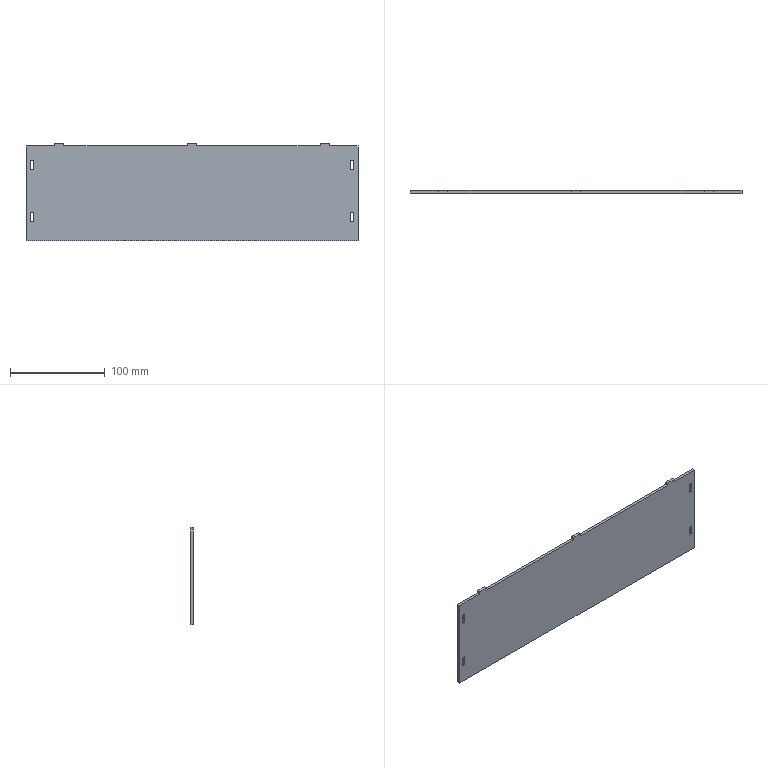Part | SolidWorks | features ICE 2, Extrusion 1 | 1 solid | 34 faces | box 350 x 3 x 103 mm | volume 104878 mm3 | plane 34
STEP:
#1=CARTESIAN_POINT('',(145.,3.,50.));
#2=VERTEX_POINT('',#1);
#3=CARTESIAN_POINT('',(175.,3.,50.));
#4=VERTEX_POINT('',#3);
#5=CARTESIAN_POINT('',(-175.,3.,50.));
#6=DIRECTION('',(1.,0.,0.));
#7=VECTOR('',#6,1000.);
#8=LINE('',#5,#7);
#9=EDGE_CURVE('',#2,#4,#8,.T.);
#10=ORIENTED_EDGE('',*,*,#9,.F.);
#11=CARTESIAN_POINT('',(145.,0.,50.));
#12=VERTEX_POINT('',#11);
#13=CARTESIAN_POINT('',(145.,-10.44,50.));
#14=DIRECTION('',(0.,1.,0.));
#15=VECTOR('',#14,1000.);
#16=LINE('',#13,#15);
#17=EDGE_CURVE('',#12,#2,#16,.T.);
#18=ORIENTED_EDGE('',*,*,#17,.F.);
#19=CARTESIAN_POINT('',(175.,0.,50.));
#20=VERTEX_POINT('',#19);
#21=CARTESIAN_POINT('',(-175.,0.,50.));
#22=DIRECTION('',(1.,0.,0.));
#23=VECTOR('',#22,1000.);
#24=LINE('',#21,#23);
#25=EDGE_CURVE('',#12,#20,#24,.T.);
#26=ORIENTED_EDGE('',*,*,#25,.T.);
#27=CARTESIAN_POINT('',(175.,3.,50.));
#28=DIRECTION('',(0.,-1.,0.));
#29=VECTOR('',#28,1000.);
#30=LINE('',#27,#29);
#31=EDGE_CURVE('',#4,#20,#30,.T.);
#32=ORIENTED_EDGE('',*,*,#31,.F.);
#33=EDGE_LOOP('',(#10,#18,#26,#32));
#34=FACE_OUTER_BOUND('',#33,.T.);
#35=CARTESIAN_POINT('',(-175.,3.,50.));
#36=DIRECTION('',(0.,0.,-1.));
#37=DIRECTION('',(-1.,0.,0.));
#38=AXIS2_PLACEMENT_3D('',#35,#36,#37);
#39=PLANE('',#38);
#40=ADVANCED_FACE('',(#34),#39,.F.);
#41=CARTESIAN_POINT('',(-135.,0.,50.));
#42=VERTEX_POINT('',#41);
#43=CARTESIAN_POINT('',(-5.,0.,50.));
#44=VERTEX_POINT('',#43);
#45=CARTESIAN_POINT('',(-175.,0.,50.));
#46=DIRECTION('',(1.,0.,0.));
#47=VECTOR('',#46,1000.);
#48=LINE('',#45,#47);
#49=EDGE_CURVE('',#42,#44,#48,.T.);
#50=ORIENTED_EDGE('',*,*,#49,.T.);
#51=CARTESIAN_POINT('',(-5.,3.,50.));
#52=VERTEX_POINT('',#51);
#53=CARTESIAN_POINT('',(-5.,-10.44,50.));
#54=DIRECTION('',(0.,1.,0.));
#55=VECTOR('',#54,1000.);
#56=LINE('',#53,#55);
#57=EDGE_CURVE('',#44,#52,#56,.T.);
#58=ORIENTED_EDGE('',*,*,#57,.T.);
#59=CARTESIAN_POINT('',(-135.,3.,50.));
#60=VERTEX_POINT('',#59);
#61=CARTESIAN_POINT('',(-175.,3.,50.));
#62=DIRECTION('',(1.,0.,0.));
#63=VECTOR('',#62,1000.);
#64=LINE('',#61,#63);
#65=EDGE_CURVE('',#60,#52,#64,.T.);
#66=ORIENTED_EDGE('',*,*,#65,.F.);
#67=CARTESIAN_POINT('',(-135.,-10.44,50.));
#68=DIRECTION('',(0.,1.,0.));
#69=VECTOR('',#68,1000.);
#70=LINE('',#67,#69);
#71=EDGE_CURVE('',#42,#60,#70,.T.);
#72=ORIENTED_EDGE('',*,*,#71,.F.);
#73=EDGE_LOOP('',(#50,#58,#66,#72));
#74=FACE_OUTER_BOUND('',#73,.T.);
#75=CARTESIAN_POINT('',(-175.,3.,50.));
#76=DIRECTION('',(0.,0.,-1.));
#77=DIRECTION('',(-1.,0.,0.));
#78=AXIS2_PLACEMENT_3D('',#75,#76,#77);
#79=PLANE('',#78);
#80=ADVANCED_FACE('',(#74),#79,.F.);
#81=CARTESIAN_POINT('',(5.,0.,50.));
#82=VERTEX_POINT('',#81);
#83=CARTESIAN_POINT('',(135.,0.,50.));
#84=VERTEX_POINT('',#83);
#85=CARTESIAN_POINT('',(-175.,0.,50.));
#86=DIRECTION('',(1.,0.,0.));
#87=VECTOR('',#86,1000.);
#88=LINE('',#85,#87);
#89=EDGE_CURVE('',#82,#84,#88,.T.);
#90=ORIENTED_EDGE('',*,*,#89,.T.);
#91=CARTESIAN_POINT('',(135.,3.,50.));
#92=VERTEX_POINT('',#91);
#93=CARTESIAN_POINT('',(135.,-10.44,50.));
#94=DIRECTION('',(0.,1.,0.));
#95=VECTOR('',#94,1000.);
#96=LINE('',#93,#95);
#97=EDGE_CURVE('',#84,#92,#96,.T.);
#98=ORIENTED_EDGE('',*,*,#97,.T.);
#99=CARTESIAN_POINT('',(5.,3.,50.));
#100=VERTEX_POINT('',#99);
#101=CARTESIAN_POINT('',(-175.,3.,50.));
#102=DIRECTION('',(1.,0.,0.));
#103=VECTOR('',#102,1000.);
#104=LINE('',#101,#103);
#105=EDGE_CURVE('',#100,#92,#104,.T.);
#106=ORIENTED_EDGE('',*,*,#105,.F.);
#107=CARTESIAN_POINT('',(5.,-10.44,50.));
#108=DIRECTION('',(0.,1.,0.));
#109=VECTOR('',#108,1000.);
#110=LINE('',#107,#109);
#111=EDGE_CURVE('',#82,#100,#110,.T.);
#112=ORIENTED_EDGE('',*,*,#111,.F.);
#113=EDGE_LOOP('',(#90,#98,#106,#112));
#114=FACE_OUTER_BOUND('',#113,.T.);
#115=CARTESIAN_POINT('',(-175.,3.,50.));
#116=DIRECTION('',(0.,0.,-1.));
#117=DIRECTION('',(-1.,0.,0.));
#118=AXIS2_PLACEMENT_3D('',#115,#116,#117);
#119=PLANE('',#118);
#120=ADVANCED_FACE('',(#114),#119,.F.);
#121=CARTESIAN_POINT('',(175.,0.,-50.));
#122=VERTEX_POINT('',#121);
#123=CARTESIAN_POINT('',(175.,0.,50.));
#124=DIRECTION('',(0.,0.,-1.));
#125=VECTOR('',#124,1000.);
#126=LINE('',#123,#125);
#127=EDGE_CURVE('',#20,#122,#126,.T.);
#128=ORIENTED_EDGE('',*,*,#127,.T.);
#129=CARTESIAN_POINT('',(175.,3.,-50.));
#130=VERTEX_POINT('',#129);
#131=CARTESIAN_POINT('',(175.,3.,-50.));
#132=DIRECTION('',(0.,-1.,0.));
#133=VECTOR('',#132,1000.);
#134=LINE('',#131,#133);
#135=EDGE_CURVE('',#130,#122,#134,.T.);
#136=ORIENTED_EDGE('',*,*,#135,.F.);
#137=CARTESIAN_POINT('',(175.,3.,50.));
#138=DIRECTION('',(0.,0.,-1.));
#139=VECTOR('',#138,1000.);
#140=LINE('',#137,#139);
#141=EDGE_CURVE('',#4,#130,#140,.T.);
#142=ORIENTED_EDGE('',*,*,#141,.F.);
#143=ORIENTED_EDGE('',*,*,#31,.T.);
#144=EDGE_LOOP('',(#128,#136,#142,#143));
#145=FACE_OUTER_BOUND('',#144,.T.);
#146=CARTESIAN_POINT('',(175.,3.,50.));
#147=DIRECTION('',(-1.,0.,0.));
#148=DIRECTION('',(0.,0.,1.));
#149=AXIS2_PLACEMENT_3D('',#146,#147,#148);
#150=PLANE('',#149);
#151=ADVANCED_FACE('',(#145),#150,.F.);
#152=CARTESIAN_POINT('',(-175.,0.,-50.));
#153=VERTEX_POINT('',#152);
#154=CARTESIAN_POINT('',(-175.,0.,-50.));
#155=DIRECTION('',(-1.,0.,0.));
#156=VECTOR('',#155,1000.);
#157=LINE('',#154,#156);
#158=EDGE_CURVE('',#122,#153,#157,.T.);
#159=ORIENTED_EDGE('',*,*,#158,.T.);
#160=CARTESIAN_POINT('',(-175.,3.,-50.));
#161=VERTEX_POINT('',#160);
#162=CARTESIAN_POINT('',(-175.,3.,-50.));
#163=DIRECTION('',(0.,-1.,0.));
#164=VECTOR('',#163,1000.);
#165=LINE('',#162,#164);
#166=EDGE_CURVE('',#161,#153,#165,.T.);
#167=ORIENTED_EDGE('',*,*,#166,.F.);
#168=CARTESIAN_POINT('',(-175.,3.,-50.));
#169=DIRECTION('',(-1.,0.,0.));
#170=VECTOR('',#169,1000.);
#171=LINE('',#168,#170);
#172=EDGE_CURVE('',#130,#161,#171,.T.);
#173=ORIENTED_EDGE('',*,*,#172,.F.);
#174=ORIENTED_EDGE('',*,*,#135,.T.);
#175=EDGE_LOOP('',(#159,#167,#173,#174));
#176=FACE_OUTER_BOUND('',#175,.T.);
#177=CARTESIAN_POINT('',(-175.,3.,-50.));
#178=DIRECTION('',(0.,0.,1.));
#179=DIRECTION('',(1.,0.,0.));
#180=AXIS2_PLACEMENT_3D('',#177,#178,#179);
#181=PLANE('',#180);
#182=ADVANCED_FACE('',(#176),#181,.F.);
#183=CARTESIAN_POINT('',(-175.,0.,50.));
#184=VERTEX_POINT('',#183);
#185=CARTESIAN_POINT('',(-175.,0.,50.));
#186=DIRECTION('',(0.,0.,1.));
#187=VECTOR('',#186,1000.);
#188=LINE('',#185,#187);
#189=EDGE_CURVE('',#153,#184,#188,.T.);
#190=ORIENTED_EDGE('',*,*,#189,.T.);
#191=CARTESIAN_POINT('',(-175.,3.,50.));
#192=VERTEX_POINT('',#191);
#193=CARTESIAN_POINT('',(-175.,3.,50.));
#194=DIRECTION('',(0.,-1.,0.));
#195=VECTOR('',#194,1000.);
#196=LINE('',#193,#195);
#197=EDGE_CURVE('',#192,#184,#196,.T.);
#198=ORIENTED_EDGE('',*,*,#197,.F.);
#199=CARTESIAN_POINT('',(-175.,3.,50.));
#200=DIRECTION('',(0.,0.,1.));
#201=VECTOR('',#200,1000.);
#202=LINE('',#199,#201);
#203=EDGE_CURVE('',#161,#192,#202,.T.);
#204=ORIENTED_EDGE('',*,*,#203,.F.);
#205=ORIENTED_EDGE('',*,*,#166,.T.);
#206=EDGE_LOOP('',(#190,#198,#204,#205));
#207=FACE_OUTER_BOUND('',#206,.T.);
#208=CARTESIAN_POINT('',(-175.,3.,50.));
#209=DIRECTION('',(1.,0.,0.));
#210=DIRECTION('',(0.,0.,-1.));
#211=AXIS2_PLACEMENT_3D('',#208,#209,#210);
#212=PLANE('',#211);
#213=ADVANCED_FACE('',(#207),#212,.F.);
#214=CARTESIAN_POINT('',(-145.,0.,50.));
#215=VERTEX_POINT('',#214);
#216=CARTESIAN_POINT('',(-175.,0.,50.));
#217=DIRECTION('',(1.,0.,0.));
#218=VECTOR('',#217,1000.);
#219=LINE('',#216,#218);
#220=EDGE_CURVE('',#184,#215,#219,.T.);
#221=ORIENTED_EDGE('',*,*,#220,.T.);
#222=CARTESIAN_POINT('',(-145.,3.,50.));
#223=VERTEX_POINT('',#222);
#224=CARTESIAN_POINT('',(-145.,-10.44,50.));
#225=DIRECTION('',(0.,1.,0.));
#226=VECTOR('',#225,1000.);
#227=LINE('',#224,#226);
#228=EDGE_CURVE('',#215,#223,#227,.T.);
#229=ORIENTED_EDGE('',*,*,#228,.T.);
#230=CARTESIAN_POINT('',(-175.,3.,50.));
#231=DIRECTION('',(1.,0.,0.));
#232=VECTOR('',#231,1000.);
#233=LINE('',#230,#232);
#234=EDGE_CURVE('',#192,#223,#233,.T.);
#235=ORIENTED_EDGE('',*,*,#234,.F.);
#236=ORIENTED_EDGE('',*,*,#197,.T.);
#237=EDGE_LOOP('',(#221,#229,#235,#236));
#238=FACE_OUTER_BOUND('',#237,.T.);
#239=CARTESIAN_POINT('',(-175.,3.,50.));
#240=DIRECTION('',(0.,0.,-1.));
#241=DIRECTION('',(-1.,0.,0.));
#242=AXIS2_PLACEMENT_3D('',#239,#240,#241);
#243=PLANE('',#242);
#244=ADVANCED_FACE('',(#238),#243,.F.);
#245=CARTESIAN_POINT('',(167.4,3.,-30.1));
#246=VERTEX_POINT('',#245);
#247=CARTESIAN_POINT('',(167.4,3.,-19.9));
#248=VERTEX_POINT('',#247);
#249=CARTESIAN_POINT('',(167.4,3.,-30.1));
#250=DIRECTION('',(0.,0.,1.));
#251=VECTOR('',#250,1000.);
#252=LINE('',#249,#251);
#253=EDGE_CURVE('',#246,#248,#252,.T.);
#254=ORIENTED_EDGE('',*,*,#253,.F.);
#255=CARTESIAN_POINT('',(170.6,3.,-30.1));
#256=VERTEX_POINT('',#255);
#257=CARTESIAN_POINT('',(170.6,3.,-30.1));
#258=DIRECTION('',(-1.,0.,0.));
#259=VECTOR('',#258,1000.);
#260=LINE('',#257,#259);
#261=EDGE_CURVE('',#256,#246,#260,.T.);
#262=ORIENTED_EDGE('',*,*,#261,.F.);
#263=CARTESIAN_POINT('',(170.6,3.,-19.9));
#264=VERTEX_POINT('',#263);
#265=CARTESIAN_POINT('',(170.6,3.,-30.1));
#266=DIRECTION('',(0.,0.,-1.));
#267=VECTOR('',#266,1000.);
#268=LINE('',#265,#267);
#269=EDGE_CURVE('',#264,#256,#268,.T.);
#270=ORIENTED_EDGE('',*,*,#269,.F.);
#271=CARTESIAN_POINT('',(170.6,3.,-19.9));
#272=DIRECTION('',(1.,0.,0.));
#273=VECTOR('',#272,1000.);
#274=LINE('',#271,#273);
#275=EDGE_CURVE('',#248,#264,#274,.T.);
#276=ORIENTED_EDGE('',*,*,#275,.F.);
#277=EDGE_LOOP('',(#254,#262,#270,#276));
#278=FACE_BOUND('',#277,.T.);
#279=CARTESIAN_POINT('',(167.4,3.,24.9));
#280=VERTEX_POINT('',#279);
#281=CARTESIAN_POINT('',(167.4,3.,35.1));
#282=VERTEX_POINT('',#281);
#283=CARTESIAN_POINT('',(167.4,3.,24.9));
#284=DIRECTION('',(0.,0.,1.));
#285=VECTOR('',#284,1000.);
#286=LINE('',#283,#285);
#287=EDGE_CURVE('',#280,#282,#286,.T.);
#288=ORIENTED_EDGE('',*,*,#287,.F.);
#289=CARTESIAN_POINT('',(170.6,3.,24.9));
#290=VERTEX_POINT('',#289);
#291=CARTESIAN_POINT('',(170.6,3.,24.9));
#292=DIRECTION('',(-1.,0.,0.));
#293=VECTOR('',#292,1000.);
#294=LINE('',#291,#293);
#295=EDGE_CURVE('',#290,#280,#294,.T.);
#296=ORIENTED_EDGE('',*,*,#295,.F.);
#297=CARTESIAN_POINT('',(170.6,3.,35.1));
#298=VERTEX_POINT('',#297);
#299=CARTESIAN_POINT('',(170.6,3.,24.9));
#300=DIRECTION('',(0.,0.,-1.));
#301=VECTOR('',#300,1000.);
#302=LINE('',#299,#301);
#303=EDGE_CURVE('',#298,#290,#302,.T.);
#304=ORIENTED_EDGE('',*,*,#303,.F.);
#305=CARTESIAN_POINT('',(170.6,3.,35.1));
#306=DIRECTION('',(1.,0.,0.));
#307=VECTOR('',#306,1000.);
#308=LINE('',#305,#307);
#309=EDGE_CURVE('',#282,#298,#308,.T.);
#310=ORIENTED_EDGE('',*,*,#309,.F.);
#311=EDGE_LOOP('',(#288,#296,#304,#310));
#312=FACE_BOUND('',#311,.T.);
#313=CARTESIAN_POINT('',(-170.6,3.,35.1));
#314=VERTEX_POINT('',#313);
#315=CARTESIAN_POINT('',(-167.4,3.,35.1));
#316=VERTEX_POINT('',#315);
#317=CARTESIAN_POINT('',(-170.6,3.,35.1));
#318=DIRECTION('',(1.,0.,0.));
#319=VECTOR('',#318,1000.);
#320=LINE('',#317,#319);
#321=EDGE_CURVE('',#314,#316,#320,.T.);
#322=ORIENTED_EDGE('',*,*,#321,.F.);
#323=CARTESIAN_POINT('',(-170.6,3.,24.9));
#324=VERTEX_POINT('',#323);
#325=CARTESIAN_POINT('',(-170.6,3.,24.9));
#326=DIRECTION('',(0.,0.,1.));
#327=VECTOR('',#326,1000.);
#328=LINE('',#325,#327);
#329=EDGE_CURVE('',#324,#314,#328,.T.);
#330=ORIENTED_EDGE('',*,*,#329,.F.);
#331=CARTESIAN_POINT('',(-167.4,3.,24.9));
#332=VERTEX_POINT('',#331);
#333=CARTESIAN_POINT('',(-170.6,3.,24.9));
#334=DIRECTION('',(-1.,0.,0.));
#335=VECTOR('',#334,1000.);
#336=LINE('',#333,#335);
#337=EDGE_CURVE('',#332,#324,#336,.T.);
#338=ORIENTED_EDGE('',*,*,#337,.F.);
#339=CARTESIAN_POINT('',(-167.4,3.,24.9));
#340=DIRECTION('',(0.,0.,-1.));
#341=VECTOR('',#340,1000.);
#342=LINE('',#339,#341);
#343=EDGE_CURVE('',#316,#332,#342,.T.);
#344=ORIENTED_EDGE('',*,*,#343,.F.);
#345=EDGE_LOOP('',(#322,#330,#338,#344));
#346=FACE_BOUND('',#345,.T.);
#347=CARTESIAN_POINT('',(-170.6,3.,-19.9));
#348=VERTEX_POINT('',#347);
#349=CARTESIAN_POINT('',(-167.4,3.,-19.9));
#350=VERTEX_POINT('',#349);
#351=CARTESIAN_POINT('',(-170.6,3.,-19.9));
#352=DIRECTION('',(1.,0.,0.));
#353=VECTOR('',#352,1000.);
#354=LINE('',#351,#353);
#355=EDGE_CURVE('',#348,#350,#354,.T.);
#356=ORIENTED_EDGE('',*,*,#355,.F.);
#357=CARTESIAN_POINT('',(-170.6,3.,-30.1));
#358=VERTEX_POINT('',#357);
#359=CARTESIAN_POINT('',(-170.6,3.,-30.1));
#360=DIRECTION('',(0.,0.,1.));
#361=VECTOR('',#360,1000.);
#362=LINE('',#359,#361);
#363=EDGE_CURVE('',#358,#348,#362,.T.);
#364=ORIENTED_EDGE('',*,*,#363,.F.);
#365=CARTESIAN_POINT('',(-167.4,3.,-30.1));
#366=VERTEX_POINT('',#365);
#367=CARTESIAN_POINT('',(-170.6,3.,-30.1));
#368=DIRECTION('',(-1.,0.,0.));
#369=VECTOR('',#368,1000.);
#370=LINE('',#367,#369);
#371=EDGE_CURVE('',#366,#358,#370,.T.);
#372=ORIENTED_EDGE('',*,*,#371,.F.);
#373=CARTESIAN_POINT('',(-167.4,3.,-30.1));
#374=DIRECTION('',(0.,0.,-1.));
#375=VECTOR('',#374,1000.);
#376=LINE('',#373,#375);
#377=EDGE_CURVE('',#350,#366,#376,.T.);
#378=ORIENTED_EDGE('',*,*,#377,.F.);
#379=EDGE_LOOP('',(#356,#364,#372,#378));
#380=FACE_BOUND('',#379,.T.);
#381=ORIENTED_EDGE('',*,*,#141,.T.);
#382=ORIENTED_EDGE('',*,*,#172,.T.);
#383=ORIENTED_EDGE('',*,*,#203,.T.);
#384=ORIENTED_EDGE('',*,*,#234,.T.);
#385=CARTESIAN_POINT('',(-145.,3.,53.));
#386=VERTEX_POINT('',#385);
#387=CARTESIAN_POINT('',(-145.,3.,50.));
#388=DIRECTION('',(0.,0.,1.));
#389=VECTOR('',#388,1000.);
#390=LINE('',#387,#389);
#391=EDGE_CURVE('',#223,#386,#390,.T.);
#392=ORIENTED_EDGE('',*,*,#391,.T.);
#393=CARTESIAN_POINT('',(-135.,3.,53.));
#394=VERTEX_POINT('',#393);
#395=CARTESIAN_POINT('',(-145.,3.,53.));
#396=DIRECTION('',(1.,0.,0.));
#397=VECTOR('',#396,1000.);
#398=LINE('',#395,#397);
#399=EDGE_CURVE('',#386,#394,#398,.T.);
#400=ORIENTED_EDGE('',*,*,#399,.T.);
#401=CARTESIAN_POINT('',(-135.,3.,50.));
#402=DIRECTION('',(0.,0.,-1.));
#403=VECTOR('',#402,1000.);
#404=LINE('',#401,#403);
#405=EDGE_CURVE('',#394,#60,#404,.T.);
#406=ORIENTED_EDGE('',*,*,#405,.T.);
#407=ORIENTED_EDGE('',*,*,#65,.T.);
#408=CARTESIAN_POINT('',(-5.,3.,53.));
#409=VERTEX_POINT('',#408);
#410=CARTESIAN_POINT('',(-5.,3.,53.));
#411=DIRECTION('',(0.,0.,1.));
#412=VECTOR('',#411,1000.);
#413=LINE('',#410,#412);
#414=EDGE_CURVE('',#52,#409,#413,.T.);
#415=ORIENTED_EDGE('',*,*,#414,.T.);
#416=CARTESIAN_POINT('',(5.,3.,53.));
#417=VERTEX_POINT('',#416);
#418=CARTESIAN_POINT('',(-5.,3.,53.));
#419=DIRECTION('',(1.,0.,0.));
#420=VECTOR('',#419,1000.);
#421=LINE('',#418,#420);
#422=EDGE_CURVE('',#409,#417,#421,.T.);
#423=ORIENTED_EDGE('',*,*,#422,.T.);
#424=CARTESIAN_POINT('',(5.,3.,53.));
#425=DIRECTION('',(0.,0.,-1.));
#426=VECTOR('',#425,1000.);
#427=LINE('',#424,#426);
#428=EDGE_CURVE('',#417,#100,#427,.T.);
#429=ORIENTED_EDGE('',*,*,#428,.T.);
#430=ORIENTED_EDGE('',*,*,#105,.T.);
#431=CARTESIAN_POINT('',(135.,3.,53.));
#432=VERTEX_POINT('',#431);
#433=CARTESIAN_POINT('',(135.,3.,50.));
#434=DIRECTION('',(0.,0.,1.));
#435=VECTOR('',#434,1000.);
#436=LINE('',#433,#435);
#437=EDGE_CURVE('',#92,#432,#436,.T.);
#438=ORIENTED_EDGE('',*,*,#437,.T.);
#439=CARTESIAN_POINT('',(145.,3.,53.));
#440=VERTEX_POINT('',#439);
#441=CARTESIAN_POINT('',(135.,3.,53.));
#442=DIRECTION('',(1.,0.,0.));
#443=VECTOR('',#442,1000.);
#444=LINE('',#441,#443);
#445=EDGE_CURVE('',#432,#440,#444,.T.);
#446=ORIENTED_EDGE('',*,*,#445,.T.);
#447=CARTESIAN_POINT('',(145.,3.,50.));
#448=DIRECTION('',(0.,0.,-1.));
#449=VECTOR('',#448,1000.);
#450=LINE('',#447,#449);
#451=EDGE_CURVE('',#440,#2,#450,.T.);
#452=ORIENTED_EDGE('',*,*,#451,.T.);
#453=ORIENTED_EDGE('',*,*,#9,.T.);
#454=EDGE_LOOP('',(#381,#382,#383,#384,#392,#400,#406,#407,#415,#423,#429,#430,#438,#446,#452,#453));
#455=FACE_OUTER_BOUND('',#454,.T.);
#456=CARTESIAN_POINT('',(0.,3.,0.));
#457=DIRECTION('',(0.,-1.,0.));
#458=DIRECTION('',(0.,0.,-1.));
#459=AXIS2_PLACEMENT_3D('',#456,#457,#458);
#460=PLANE('',#459);
#461=ADVANCED_FACE('',(#278,#312,#346,#380,#455),#460,.F.);
#462=CARTESIAN_POINT('',(170.6,0.,-30.1));
#463=VERTEX_POINT('',#462);
#464=CARTESIAN_POINT('',(167.4,0.,-30.1));
#465=VERTEX_POINT('',#464);
#466=CARTESIAN_POINT('',(170.6,0.,-30.1));
#467=DIRECTION('',(-1.,0.,0.));
#468=VECTOR('',#467,1000.);
#469=LINE('',#466,#468);
#470=EDGE_CURVE('',#463,#465,#469,.T.);
#471=ORIENTED_EDGE('',*,*,#470,.T.);
#472=CARTESIAN_POINT('',(167.4,0.,-19.9));
#473=VERTEX_POINT('',#472);
#474=CARTESIAN_POINT('',(167.4,0.,-30.1));
#475=DIRECTION('',(0.,0.,1.));
#476=VECTOR('',#475,1000.);
#477=LINE('',#474,#476);
#478=EDGE_CURVE('',#465,#473,#477,.T.);
#479=ORIENTED_EDGE('',*,*,#478,.T.);
#480=CARTESIAN_POINT('',(170.6,0.,-19.9));
#481=VERTEX_POINT('',#480);
#482=CARTESIAN_POINT('',(170.6,0.,-19.9));
#483=DIRECTION('',(1.,0.,0.));
#484=VECTOR('',#483,1000.);
#485=LINE('',#482,#484);
#486=EDGE_CURVE('',#473,#481,#485,.T.);
#487=ORIENTED_EDGE('',*,*,#486,.T.);
#488=CARTESIAN_POINT('',(170.6,0.,-30.1));
#489=DIRECTION('',(0.,0.,-1.));
#490=VECTOR('',#489,1000.);
#491=LINE('',#488,#490);
#492=EDGE_CURVE('',#481,#463,#491,.T.);
#493=ORIENTED_EDGE('',*,*,#492,.T.);
#494=EDGE_LOOP('',(#471,#479,#487,#493));
#495=FACE_BOUND('',#494,.T.);
#496=CARTESIAN_POINT('',(170.6,0.,24.9));
#497=VERTEX_POINT('',#496);
#498=CARTESIAN_POINT('',(167.4,0.,24.9));
#499=VERTEX_POINT('',#498);
#500=CARTESIAN_POINT('',(170.6,0.,24.9));
#501=DIRECTION('',(-1.,0.,0.));
#502=VECTOR('',#501,1000.);
#503=LINE('',#500,#502);
#504=EDGE_CURVE('',#497,#499,#503,.T.);
#505=ORIENTED_EDGE('',*,*,#504,.T.);
#506=CARTESIAN_POINT('',(167.4,0.,35.1));
#507=VERTEX_POINT('',#506);
#508=CARTESIAN_POINT('',(167.4,0.,24.9));
#509=DIRECTION('',(0.,0.,1.));
#510=VECTOR('',#509,1000.);
#511=LINE('',#508,#510);
#512=EDGE_CURVE('',#499,#507,#511,.T.);
#513=ORIENTED_EDGE('',*,*,#512,.T.);
#514=CARTESIAN_POINT('',(170.6,0.,35.1));
#515=VERTEX_POINT('',#514);
#516=CARTESIAN_POINT('',(170.6,0.,35.1));
#517=DIRECTION('',(1.,0.,0.));
#518=VECTOR('',#517,1000.);
#519=LINE('',#516,#518);
#520=EDGE_CURVE('',#507,#515,#519,.T.);
#521=ORIENTED_EDGE('',*,*,#520,.T.);
#522=CARTESIAN_POINT('',(170.6,0.,24.9));
#523=DIRECTION('',(0.,0.,-1.));
#524=VECTOR('',#523,1000.);
#525=LINE('',#522,#524);
#526=EDGE_CURVE('',#515,#497,#525,.T.);
#527=ORIENTED_EDGE('',*,*,#526,.T.);
#528=EDGE_LOOP('',(#505,#513,#521,#527));
#529=FACE_BOUND('',#528,.T.);
#530=CARTESIAN_POINT('',(-170.6,0.,24.9));
#531=VERTEX_POINT('',#530);
#532=CARTESIAN_POINT('',(-170.6,0.,35.1));
#533=VERTEX_POINT('',#532);
#534=CARTESIAN_POINT('',(-170.6,0.,24.9));
#535=DIRECTION('',(0.,0.,1.));
#536=VECTOR('',#535,1000.);
#537=LINE('',#534,#536);
#538=EDGE_CURVE('',#531,#533,#537,.T.);
#539=ORIENTED_EDGE('',*,*,#538,.T.);
#540=CARTESIAN_POINT('',(-167.4,0.,35.1));
#541=VERTEX_POINT('',#540);
#542=CARTESIAN_POINT('',(-170.6,0.,35.1));
#543=DIRECTION('',(1.,0.,0.));
#544=VECTOR('',#543,1000.);
#545=LINE('',#542,#544);
#546=EDGE_CURVE('',#533,#541,#545,.T.);
#547=ORIENTED_EDGE('',*,*,#546,.T.);
#548=CARTESIAN_POINT('',(-167.4,0.,24.9));
#549=VERTEX_POINT('',#548);
#550=CARTESIAN_POINT('',(-167.4,0.,24.9));
#551=DIRECTION('',(0.,0.,-1.));
#552=VECTOR('',#551,1000.);
#553=LINE('',#550,#552);
#554=EDGE_CURVE('',#541,#549,#553,.T.);
#555=ORIENTED_EDGE('',*,*,#554,.T.);
#556=CARTESIAN_POINT('',(-170.6,0.,24.9));
#557=DIRECTION('',(-1.,0.,0.));
#558=VECTOR('',#557,1000.);
#559=LINE('',#556,#558);
#560=EDGE_CURVE('',#549,#531,#559,.T.);
#561=ORIENTED_EDGE('',*,*,#560,.T.);
#562=EDGE_LOOP('',(#539,#547,#555,#561));
#563=FACE_BOUND('',#562,.T.);
#564=CARTESIAN_POINT('',(-170.6,0.,-30.1));
#565=VERTEX_POINT('',#564);
#566=CARTESIAN_POINT('',(-170.6,0.,-19.9));
#567=VERTEX_POINT('',#566);
#568=CARTESIAN_POINT('',(-170.6,0.,-30.1));
#569=DIRECTION('',(0.,0.,1.));
#570=VECTOR('',#569,1000.);
#571=LINE('',#568,#570);
#572=EDGE_CURVE('',#565,#567,#571,.T.);
#573=ORIENTED_EDGE('',*,*,#572,.T.);
#574=CARTESIAN_POINT('',(-167.4,0.,-19.9));
#575=VERTEX_POINT('',#574);
#576=CARTESIAN_POINT('',(-170.6,0.,-19.9));
#577=DIRECTION('',(1.,0.,0.));
#578=VECTOR('',#577,1000.);
#579=LINE('',#576,#578);
#580=EDGE_CURVE('',#567,#575,#579,.T.);
#581=ORIENTED_EDGE('',*,*,#580,.T.);
#582=CARTESIAN_POINT('',(-167.4,0.,-30.1));
#583=VERTEX_POINT('',#582);
#584=CARTESIAN_POINT('',(-167.4,0.,-30.1));
#585=DIRECTION('',(0.,0.,-1.));
#586=VECTOR('',#585,1000.);
#587=LINE('',#584,#586);
#588=EDGE_CURVE('',#575,#583,#587,.T.);
#589=ORIENTED_EDGE('',*,*,#588,.T.);
#590=CARTESIAN_POINT('',(-170.6,0.,-30.1));
#591=DIRECTION('',(-1.,0.,0.));
#592=VECTOR('',#591,1000.);
#593=LINE('',#590,#592);
#594=EDGE_CURVE('',#583,#565,#593,.T.);
#595=ORIENTED_EDGE('',*,*,#594,.T.);
#596=EDGE_LOOP('',(#573,#581,#589,#595));
#597=FACE_BOUND('',#596,.T.);
#598=ORIENTED_EDGE('',*,*,#127,.F.);
#599=ORIENTED_EDGE('',*,*,#25,.F.);
#600=CARTESIAN_POINT('',(145.,0.,53.));
#601=VERTEX_POINT('',#600);
#602=CARTESIAN_POINT('',(145.,0.,50.));
#603=DIRECTION('',(0.,0.,-1.));
#604=VECTOR('',#603,1000.);
#605=LINE('',#602,#604);
#606=EDGE_CURVE('',#601,#12,#605,.T.);
#607=ORIENTED_EDGE('',*,*,#606,.F.);
#608=CARTESIAN_POINT('',(135.,0.,53.));
#609=VERTEX_POINT('',#608);
#610=CARTESIAN_POINT('',(135.,0.,53.));
#611=DIRECTION('',(1.,0.,0.));
#612=VECTOR('',#611,1000.);
#613=LINE('',#610,#612);
#614=EDGE_CURVE('',#609,#601,#613,.T.);
#615=ORIENTED_EDGE('',*,*,#614,.F.);
#616=CARTESIAN_POINT('',(135.,0.,50.));
#617=DIRECTION('',(0.,0.,1.));
#618=VECTOR('',#617,1000.);
#619=LINE('',#616,#618);
#620=EDGE_CURVE('',#84,#609,#619,.T.);
#621=ORIENTED_EDGE('',*,*,#620,.F.);
#622=ORIENTED_EDGE('',*,*,#89,.F.);
#623=CARTESIAN_POINT('',(5.,0.,53.));
#624=VERTEX_POINT('',#623);
#625=CARTESIAN_POINT('',(5.,0.,53.));
#626=DIRECTION('',(0.,0.,-1.));
#627=VECTOR('',#626,1000.);
#628=LINE('',#625,#627);
#629=EDGE_CURVE('',#624,#82,#628,.T.);
#630=ORIENTED_EDGE('',*,*,#629,.F.);
#631=CARTESIAN_POINT('',(-5.,0.,53.));
#632=VERTEX_POINT('',#631);
#633=CARTESIAN_POINT('',(-5.,0.,53.));
#634=DIRECTION('',(1.,0.,0.));
#635=VECTOR('',#634,1000.);
#636=LINE('',#633,#635);
#637=EDGE_CURVE('',#632,#624,#636,.T.);
#638=ORIENTED_EDGE('',*,*,#637,.F.);
#639=CARTESIAN_POINT('',(-5.,0.,53.));
#640=DIRECTION('',(0.,0.,1.));
#641=VECTOR('',#640,1000.);
#642=LINE('',#639,#641);
#643=EDGE_CURVE('',#44,#632,#642,.T.);
#644=ORIENTED_EDGE('',*,*,#643,.F.);
#645=ORIENTED_EDGE('',*,*,#49,.F.);
#646=CARTESIAN_POINT('',(-135.,0.,53.));
#647=VERTEX_POINT('',#646);
#648=CARTESIAN_POINT('',(-135.,0.,50.));
#649=DIRECTION('',(0.,0.,-1.));
#650=VECTOR('',#649,1000.);
#651=LINE('',#648,#650);
#652=EDGE_CURVE('',#647,#42,#651,.T.);
#653=ORIENTED_EDGE('',*,*,#652,.F.);
#654=CARTESIAN_POINT('',(-145.,0.,53.));
#655=VERTEX_POINT('',#654);
#656=CARTESIAN_POINT('',(-145.,0.,53.));
#657=DIRECTION('',(1.,0.,0.));
#658=VECTOR('',#657,1000.);
#659=LINE('',#656,#658);
#660=EDGE_CURVE('',#655,#647,#659,.T.);
#661=ORIENTED_EDGE('',*,*,#660,.F.);
#662=CARTESIAN_POINT('',(-145.,0.,50.));
#663=DIRECTION('',(0.,0.,1.));
#664=VECTOR('',#663,1000.);
#665=LINE('',#662,#664);
#666=EDGE_CURVE('',#215,#655,#665,.T.);
#667=ORIENTED_EDGE('',*,*,#666,.F.);
#668=ORIENTED_EDGE('',*,*,#220,.F.);
#669=ORIENTED_EDGE('',*,*,#189,.F.);
#670=ORIENTED_EDGE('',*,*,#158,.F.);
#671=EDGE_LOOP('',(#598,#599,#607,#615,#621,#622,#630,#638,#644,#645,#653,#661,#667,#668,#669,#670));
#672=FACE_OUTER_BOUND('',#671,.T.);
#673=CARTESIAN_POINT('',(0.,0.,0.));
#674=DIRECTION('',(0.,-1.,0.));
#675=DIRECTION('',(0.,0.,-1.));
#676=AXIS2_PLACEMENT_3D('',#673,#674,#675);
#677=PLANE('',#676);
#678=ADVANCED_FACE('',(#495,#529,#563,#597,#672),#677,.T.);
#679=ORIENTED_EDGE('',*,*,#363,.T.);
#680=CARTESIAN_POINT('',(-170.6,0.,-19.9));
#681=DIRECTION('',(0.,1.,0.));
#682=VECTOR('',#681,1000.);
#683=LINE('',#680,#682);
#684=EDGE_CURVE('',#567,#348,#683,.T.);
#685=ORIENTED_EDGE('',*,*,#684,.F.);
#686=ORIENTED_EDGE('',*,*,#572,.F.);
#687=CARTESIAN_POINT('',(-170.6,0.,-30.1));
#688=DIRECTION('',(0.,1.,0.));
#689=VECTOR('',#688,1000.);
#690=LINE('',#687,#689);
#691=EDGE_CURVE('',#565,#358,#690,.T.);
#692=ORIENTED_EDGE('',*,*,#691,.T.);
#693=EDGE_LOOP('',(#679,#685,#686,#692));
#694=FACE_OUTER_BOUND('',#693,.T.);
#695=CARTESIAN_POINT('',(-170.6,0.,-30.1));
#696=DIRECTION('',(-1.,0.,0.));
#697=DIRECTION('',(0.,0.,1.));
#698=AXIS2_PLACEMENT_3D('',#695,#696,#697);
#699=PLANE('',#698);
#700=ADVANCED_FACE('',(#694),#699,.F.);
#701=ORIENTED_EDGE('',*,*,#371,.T.);
#702=ORIENTED_EDGE('',*,*,#691,.F.);
#703=ORIENTED_EDGE('',*,*,#594,.F.);
#704=CARTESIAN_POINT('',(-167.4,0.,-30.1));
#705=DIRECTION('',(0.,1.,0.));
#706=VECTOR('',#705,1000.);
#707=LINE('',#704,#706);
#708=EDGE_CURVE('',#583,#366,#707,.T.);
#709=ORIENTED_EDGE('',*,*,#708,.T.);
#710=EDGE_LOOP('',(#701,#702,#703,#709));
#711=FACE_OUTER_BOUND('',#710,.T.);
#712=CARTESIAN_POINT('',(-170.6,0.,-30.1));
#713=DIRECTION('',(0.,0.,-1.));
#714=DIRECTION('',(-1.,0.,0.));
#715=AXIS2_PLACEMENT_3D('',#712,#713,#714);
#716=PLANE('',#715);
#717=ADVANCED_FACE('',(#711),#716,.F.);
#718=ORIENTED_EDGE('',*,*,#377,.T.);
#719=ORIENTED_EDGE('',*,*,#708,.F.);
#720=ORIENTED_EDGE('',*,*,#588,.F.);
#721=CARTESIAN_POINT('',(-167.4,0.,-19.9));
#722=DIRECTION('',(0.,1.,0.));
#723=VECTOR('',#722,1000.);
#724=LINE('',#721,#723);
#725=EDGE_CURVE('',#575,#350,#724,.T.);
#726=ORIENTED_EDGE('',*,*,#725,.T.);
#727=EDGE_LOOP('',(#718,#719,#720,#726));
#728=FACE_OUTER_BOUND('',#727,.T.);
#729=CARTESIAN_POINT('',(-167.4,0.,-30.1));
#730=DIRECTION('',(1.,0.,0.));
#731=DIRECTION('',(0.,0.,-1.));
#732=AXIS2_PLACEMENT_3D('',#729,#730,#731);
#733=PLANE('',#732);
#734=ADVANCED_FACE('',(#728),#733,.F.);
#735=ORIENTED_EDGE('',*,*,#355,.T.);
#736=ORIENTED_EDGE('',*,*,#725,.F.);
#737=ORIENTED_EDGE('',*,*,#580,.F.);
#738=ORIENTED_EDGE('',*,*,#684,.T.);
#739=EDGE_LOOP('',(#735,#736,#737,#738));
#740=FACE_OUTER_BOUND('',#739,.T.);
#741=CARTESIAN_POINT('',(-170.6,0.,-19.9));
#742=DIRECTION('',(0.,0.,1.));
#743=DIRECTION('',(1.,0.,0.));
#744=AXIS2_PLACEMENT_3D('',#741,#742,#743);
#745=PLANE('',#744);
#746=ADVANCED_FACE('',(#740),#745,.F.);
#747=ORIENTED_EDGE('',*,*,#329,.T.);
#748=CARTESIAN_POINT('',(-170.6,0.,35.1));
#749=DIRECTION('',(0.,1.,0.));
#750=VECTOR('',#749,1000.);
#751=LINE('',#748,#750);
#752=EDGE_CURVE('',#533,#314,#751,.T.);
#753=ORIENTED_EDGE('',*,*,#752,.F.);
#754=ORIENTED_EDGE('',*,*,#538,.F.);
#755=CARTESIAN_POINT('',(-170.6,0.,24.9));
#756=DIRECTION('',(0.,1.,0.));
#757=VECTOR('',#756,1000.);
#758=LINE('',#755,#757);
#759=EDGE_CURVE('',#531,#324,#758,.T.);
#760=ORIENTED_EDGE('',*,*,#759,.T.);
#761=EDGE_LOOP('',(#747,#753,#754,#760));
#762=FACE_OUTER_BOUND('',#761,.T.);
#763=CARTESIAN_POINT('',(-170.6,0.,24.9));
#764=DIRECTION('',(-1.,0.,0.));
#765=DIRECTION('',(0.,0.,1.));
#766=AXIS2_PLACEMENT_3D('',#763,#764,#765);
#767=PLANE('',#766);
#768=ADVANCED_FACE('',(#762),#767,.F.);
#769=ORIENTED_EDGE('',*,*,#337,.T.);
#770=ORIENTED_EDGE('',*,*,#759,.F.);
#771=ORIENTED_EDGE('',*,*,#560,.F.);
#772=CARTESIAN_POINT('',(-167.4,0.,24.9));
#773=DIRECTION('',(0.,1.,0.));
#774=VECTOR('',#773,1000.);
#775=LINE('',#772,#774);
#776=EDGE_CURVE('',#549,#332,#775,.T.);
#777=ORIENTED_EDGE('',*,*,#776,.T.);
#778=EDGE_LOOP('',(#769,#770,#771,#777));
#779=FACE_OUTER_BOUND('',#778,.T.);
#780=CARTESIAN_POINT('',(-170.6,0.,24.9));
#781=DIRECTION('',(0.,0.,-1.));
#782=DIRECTION('',(-1.,0.,0.));
#783=AXIS2_PLACEMENT_3D('',#780,#781,#782);
#784=PLANE('',#783);
#785=ADVANCED_FACE('',(#779),#784,.F.);
#786=ORIENTED_EDGE('',*,*,#343,.T.);
#787=ORIENTED_EDGE('',*,*,#776,.F.);
#788=ORIENTED_EDGE('',*,*,#554,.F.);
#789=CARTESIAN_POINT('',(-167.4,0.,35.1));
#790=DIRECTION('',(0.,1.,0.));
#791=VECTOR('',#790,1000.);
#792=LINE('',#789,#791);
#793=EDGE_CURVE('',#541,#316,#792,.T.);
#794=ORIENTED_EDGE('',*,*,#793,.T.);
#795=EDGE_LOOP('',(#786,#787,#788,#794));
#796=FACE_OUTER_BOUND('',#795,.T.);
#797=CARTESIAN_POINT('',(-167.4,0.,24.9));
#798=DIRECTION('',(1.,0.,0.));
#799=DIRECTION('',(0.,0.,-1.));
#800=AXIS2_PLACEMENT_3D('',#797,#798,#799);
#801=PLANE('',#800);
#802=ADVANCED_FACE('',(#796),#801,.F.);
#803=ORIENTED_EDGE('',*,*,#321,.T.);
#804=ORIENTED_EDGE('',*,*,#793,.F.);
#805=ORIENTED_EDGE('',*,*,#546,.F.);
#806=ORIENTED_EDGE('',*,*,#752,.T.);
#807=EDGE_LOOP('',(#803,#804,#805,#806));
#808=FACE_OUTER_BOUND('',#807,.T.);
#809=CARTESIAN_POINT('',(-170.6,0.,35.1));
#810=DIRECTION('',(0.,0.,1.));
#811=DIRECTION('',(1.,0.,0.));
#812=AXIS2_PLACEMENT_3D('',#809,#810,#811);
#813=PLANE('',#812);
#814=ADVANCED_FACE('',(#808),#813,.F.);
#815=ORIENTED_EDGE('',*,*,#295,.T.);
#816=CARTESIAN_POINT('',(167.4,0.,24.9));
#817=DIRECTION('',(0.,1.,0.));
#818=VECTOR('',#817,1000.);
#819=LINE('',#816,#818);
#820=EDGE_CURVE('',#499,#280,#819,.T.);
#821=ORIENTED_EDGE('',*,*,#820,.F.);
#822=ORIENTED_EDGE('',*,*,#504,.F.);
#823=CARTESIAN_POINT('',(170.6,0.,24.9));
#824=DIRECTION('',(0.,1.,0.));
#825=VECTOR('',#824,1000.);
#826=LINE('',#823,#825);
#827=EDGE_CURVE('',#497,#290,#826,.T.);
#828=ORIENTED_EDGE('',*,*,#827,.T.);
#829=EDGE_LOOP('',(#815,#821,#822,#828));
#830=FACE_OUTER_BOUND('',#829,.T.);
#831=CARTESIAN_POINT('',(170.6,0.,24.9));
#832=DIRECTION('',(0.,0.,-1.));
#833=DIRECTION('',(-1.,0.,0.));
#834=AXIS2_PLACEMENT_3D('',#831,#832,#833);
#835=PLANE('',#834);
#836=ADVANCED_FACE('',(#830),#835,.F.);
#837=ORIENTED_EDGE('',*,*,#303,.T.);
#838=ORIENTED_EDGE('',*,*,#827,.F.);
#839=ORIENTED_EDGE('',*,*,#526,.F.);
#840=CARTESIAN_POINT('',(170.6,0.,35.1));
#841=DIRECTION('',(0.,1.,0.));
#842=VECTOR('',#841,1000.);
#843=LINE('',#840,#842);
#844=EDGE_CURVE('',#515,#298,#843,.T.);
#845=ORIENTED_EDGE('',*,*,#844,.T.);
#846=EDGE_LOOP('',(#837,#838,#839,#845));
#847=FACE_OUTER_BOUND('',#846,.T.);
#848=CARTESIAN_POINT('',(170.6,0.,24.9));
#849=DIRECTION('',(1.,0.,0.));
#850=DIRECTION('',(0.,0.,-1.));
#851=AXIS2_PLACEMENT_3D('',#848,#849,#850);
#852=PLANE('',#851);
#853=ADVANCED_FACE('',(#847),#852,.F.);
#854=ORIENTED_EDGE('',*,*,#309,.T.);
#855=ORIENTED_EDGE('',*,*,#844,.F.);
#856=ORIENTED_EDGE('',*,*,#520,.F.);
#857=CARTESIAN_POINT('',(167.4,0.,35.1));
#858=DIRECTION('',(0.,1.,0.));
#859=VECTOR('',#858,1000.);
#860=LINE('',#857,#859);
#861=EDGE_CURVE('',#507,#282,#860,.T.);
#862=ORIENTED_EDGE('',*,*,#861,.T.);
#863=EDGE_LOOP('',(#854,#855,#856,#862));
#864=FACE_OUTER_BOUND('',#863,.T.);
#865=CARTESIAN_POINT('',(170.6,0.,35.1));
#866=DIRECTION('',(0.,0.,1.));
#867=DIRECTION('',(1.,0.,0.));
#868=AXIS2_PLACEMENT_3D('',#865,#866,#867);
#869=PLANE('',#868);
#870=ADVANCED_FACE('',(#864),#869,.F.);
#871=ORIENTED_EDGE('',*,*,#287,.T.);
#872=ORIENTED_EDGE('',*,*,#861,.F.);
#873=ORIENTED_EDGE('',*,*,#512,.F.);
#874=ORIENTED_EDGE('',*,*,#820,.T.);
#875=EDGE_LOOP('',(#871,#872,#873,#874));
#876=FACE_OUTER_BOUND('',#875,.T.);
#877=CARTESIAN_POINT('',(167.4,0.,24.9));
#878=DIRECTION('',(-1.,0.,0.));
#879=DIRECTION('',(0.,0.,1.));
#880=AXIS2_PLACEMENT_3D('',#877,#878,#879);
#881=PLANE('',#880);
#882=ADVANCED_FACE('',(#876),#881,.F.);
#883=ORIENTED_EDGE('',*,*,#261,.T.);
#884=CARTESIAN_POINT('',(167.4,0.,-30.1));
#885=DIRECTION('',(0.,1.,0.));
#886=VECTOR('',#885,1000.);
#887=LINE('',#884,#886);
#888=EDGE_CURVE('',#465,#246,#887,.T.);
#889=ORIENTED_EDGE('',*,*,#888,.F.);
#890=ORIENTED_EDGE('',*,*,#470,.F.);
#891=CARTESIAN_POINT('',(170.6,0.,-30.1));
#892=DIRECTION('',(0.,1.,0.));
#893=VECTOR('',#892,1000.);
#894=LINE('',#891,#893);
#895=EDGE_CURVE('',#463,#256,#894,.T.);
#896=ORIENTED_EDGE('',*,*,#895,.T.);
#897=EDGE_LOOP('',(#883,#889,#890,#896));
#898=FACE_OUTER_BOUND('',#897,.T.);
#899=CARTESIAN_POINT('',(170.6,0.,-30.1));
#900=DIRECTION('',(0.,0.,-1.));
#901=DIRECTION('',(-1.,0.,0.));
#902=AXIS2_PLACEMENT_3D('',#899,#900,#901);
#903=PLANE('',#902);
#904=ADVANCED_FACE('',(#898),#903,.F.);
#905=ORIENTED_EDGE('',*,*,#269,.T.);
#906=ORIENTED_EDGE('',*,*,#895,.F.);
#907=ORIENTED_EDGE('',*,*,#492,.F.);
#908=CARTESIAN_POINT('',(170.6,0.,-19.9));
#909=DIRECTION('',(0.,1.,0.));
#910=VECTOR('',#909,1000.);
#911=LINE('',#908,#910);
#912=EDGE_CURVE('',#481,#264,#911,.T.);
#913=ORIENTED_EDGE('',*,*,#912,.T.);
#914=EDGE_LOOP('',(#905,#906,#907,#913));
#915=FACE_OUTER_BOUND('',#914,.T.);
#916=CARTESIAN_POINT('',(170.6,0.,-30.1));
#917=DIRECTION('',(1.,0.,0.));
#918=DIRECTION('',(0.,0.,-1.));
#919=AXIS2_PLACEMENT_3D('',#916,#917,#918);
#920=PLANE('',#919);
#921=ADVANCED_FACE('',(#915),#920,.F.);
#922=ORIENTED_EDGE('',*,*,#275,.T.);
#923=ORIENTED_EDGE('',*,*,#912,.F.);
#924=ORIENTED_EDGE('',*,*,#486,.F.);
#925=CARTESIAN_POINT('',(167.4,0.,-19.9));
#926=DIRECTION('',(0.,1.,0.));
#927=VECTOR('',#926,1000.);
#928=LINE('',#925,#927);
#929=EDGE_CURVE('',#473,#248,#928,.T.);
#930=ORIENTED_EDGE('',*,*,#929,.T.);
#931=EDGE_LOOP('',(#922,#923,#924,#930));
#932=FACE_OUTER_BOUND('',#931,.T.);
#933=CARTESIAN_POINT('',(170.6,0.,-19.9));
#934=DIRECTION('',(0.,0.,1.));
#935=DIRECTION('',(1.,0.,0.));
#936=AXIS2_PLACEMENT_3D('',#933,#934,#935);
#937=PLANE('',#936);
#938=ADVANCED_FACE('',(#932),#937,.F.);
#939=ORIENTED_EDGE('',*,*,#253,.T.);
#940=ORIENTED_EDGE('',*,*,#929,.F.);
#941=ORIENTED_EDGE('',*,*,#478,.F.);
#942=ORIENTED_EDGE('',*,*,#888,.T.);
#943=EDGE_LOOP('',(#939,#940,#941,#942));
#944=FACE_OUTER_BOUND('',#943,.T.);
#945=CARTESIAN_POINT('',(167.4,0.,-30.1));
#946=DIRECTION('',(-1.,0.,0.));
#947=DIRECTION('',(0.,0.,1.));
#948=AXIS2_PLACEMENT_3D('',#945,#946,#947);
#949=PLANE('',#948);
#950=ADVANCED_FACE('',(#944),#949,.F.);
#951=CARTESIAN_POINT('',(-145.,-10.44,53.));
#952=DIRECTION('',(0.,1.,0.));
#953=VECTOR('',#952,1000.);
#954=LINE('',#951,#953);
#955=EDGE_CURVE('',#655,#386,#954,.T.);
#956=ORIENTED_EDGE('',*,*,#955,.F.);
#957=ORIENTED_EDGE('',*,*,#660,.T.);
#958=CARTESIAN_POINT('',(-135.,-10.44,53.));
#959=DIRECTION('',(0.,1.,0.));
#960=VECTOR('',#959,1000.);
#961=LINE('',#958,#960);
#962=EDGE_CURVE('',#647,#394,#961,.T.);
#963=ORIENTED_EDGE('',*,*,#962,.T.);
#964=ORIENTED_EDGE('',*,*,#399,.F.);
#965=EDGE_LOOP('',(#956,#957,#963,#964));
#966=FACE_OUTER_BOUND('',#965,.T.);
#967=CARTESIAN_POINT('',(-145.,-10.44,53.));
#968=DIRECTION('',(0.,0.,1.));
#969=DIRECTION('',(1.,0.,0.));
#970=AXIS2_PLACEMENT_3D('',#967,#968,#969);
#971=PLANE('',#970);
#972=ADVANCED_FACE('',(#966),#971,.T.);
#973=ORIENTED_EDGE('',*,*,#962,.F.);
#974=ORIENTED_EDGE('',*,*,#652,.T.);
#975=ORIENTED_EDGE('',*,*,#71,.T.);
#976=ORIENTED_EDGE('',*,*,#405,.F.);
#977=EDGE_LOOP('',(#973,#974,#975,#976));
#978=FACE_OUTER_BOUND('',#977,.T.);
#979=CARTESIAN_POINT('',(-135.,-10.44,50.));
#980=DIRECTION('',(1.,0.,0.));
#981=DIRECTION('',(0.,0.,-1.));
#982=AXIS2_PLACEMENT_3D('',#979,#980,#981);
#983=PLANE('',#982);
#984=ADVANCED_FACE('',(#978),#983,.T.);
#985=ORIENTED_EDGE('',*,*,#228,.F.);
#986=ORIENTED_EDGE('',*,*,#666,.T.);
#987=ORIENTED_EDGE('',*,*,#955,.T.);
#988=ORIENTED_EDGE('',*,*,#391,.F.);
#989=EDGE_LOOP('',(#985,#986,#987,#988));
#990=FACE_OUTER_BOUND('',#989,.T.);
#991=CARTESIAN_POINT('',(-145.,-10.44,50.));
#992=DIRECTION('',(-1.,0.,0.));
#993=DIRECTION('',(0.,0.,1.));
#994=AXIS2_PLACEMENT_3D('',#991,#992,#993);
#995=PLANE('',#994);
#996=ADVANCED_FACE('',(#990),#995,.T.);
#997=ORIENTED_EDGE('',*,*,#57,.F.);
#998=ORIENTED_EDGE('',*,*,#643,.T.);
#999=CARTESIAN_POINT('',(-5.,-10.44,53.));
#1000=DIRECTION('',(0.,1.,0.));
#1001=VECTOR('',#1000,1000.);
#1002=LINE('',#999,#1001);
#1003=EDGE_CURVE('',#632,#409,#1002,.T.);
#1004=ORIENTED_EDGE('',*,*,#1003,.T.);
#1005=ORIENTED_EDGE('',*,*,#414,.F.);
#1006=EDGE_LOOP('',(#997,#998,#1004,#1005));
#1007=FACE_OUTER_BOUND('',#1006,.T.);
#1008=CARTESIAN_POINT('',(-5.,-10.44,53.));
#1009=DIRECTION('',(-1.,0.,0.));
#1010=DIRECTION('',(0.,0.,1.));
#1011=AXIS2_PLACEMENT_3D('',#1008,#1009,#1010);
#1012=PLANE('',#1011);
#1013=ADVANCED_FACE('',(#1007),#1012,.T.);
#1014=ORIENTED_EDGE('',*,*,#1003,.F.);
#1015=ORIENTED_EDGE('',*,*,#637,.T.);
#1016=CARTESIAN_POINT('',(5.,-10.44,53.));
#1017=DIRECTION('',(0.,1.,0.));
#1018=VECTOR('',#1017,1000.);
#1019=LINE('',#1016,#1018);
#1020=EDGE_CURVE('',#624,#417,#1019,.T.);
#1021=ORIENTED_EDGE('',*,*,#1020,.T.);
#1022=ORIENTED_EDGE('',*,*,#422,.F.);
#1023=EDGE_LOOP('',(#1014,#1015,#1021,#1022));
#1024=FACE_OUTER_BOUND('',#1023,.T.);
#1025=CARTESIAN_POINT('',(-5.,-10.44,53.));
#1026=DIRECTION('',(0.,0.,1.));
#1027=DIRECTION('',(1.,0.,0.));
#1028=AXIS2_PLACEMENT_3D('',#1025,#1026,#1027);
#1029=PLANE('',#1028);
#1030=ADVANCED_FACE('',(#1024),#1029,.T.);
#1031=ORIENTED_EDGE('',*,*,#1020,.F.);
#1032=ORIENTED_EDGE('',*,*,#629,.T.);
#1033=ORIENTED_EDGE('',*,*,#111,.T.);
#1034=ORIENTED_EDGE('',*,*,#428,.F.);
#1035=EDGE_LOOP('',(#1031,#1032,#1033,#1034));
#1036=FACE_OUTER_BOUND('',#1035,.T.);
#1037=CARTESIAN_POINT('',(5.,-10.44,53.));
#1038=DIRECTION('',(1.,0.,0.));
#1039=DIRECTION('',(0.,0.,-1.));
#1040=AXIS2_PLACEMENT_3D('',#1037,#1038,#1039);
#1041=PLANE('',#1040);
#1042=ADVANCED_FACE('',(#1036),#1041,.T.);
#1043=CARTESIAN_POINT('',(135.,-10.44,53.));
#1044=DIRECTION('',(0.,1.,0.));
#1045=VECTOR('',#1044,1000.);
#1046=LINE('',#1043,#1045);
#1047=EDGE_CURVE('',#609,#432,#1046,.T.);
#1048=ORIENTED_EDGE('',*,*,#1047,.F.);
#1049=ORIENTED_EDGE('',*,*,#614,.T.);
#1050=CARTESIAN_POINT('',(145.,-10.44,53.));
#1051=DIRECTION('',(0.,1.,0.));
#1052=VECTOR('',#1051,1000.);
#1053=LINE('',#1050,#1052);
#1054=EDGE_CURVE('',#601,#440,#1053,.T.);
#1055=ORIENTED_EDGE('',*,*,#1054,.T.);
#1056=ORIENTED_EDGE('',*,*,#445,.F.);
#1057=EDGE_LOOP('',(#1048,#1049,#1055,#1056));
#1058=FACE_OUTER_BOUND('',#1057,.T.);
#1059=CARTESIAN_POINT('',(135.,-10.44,53.));
#1060=DIRECTION('',(0.,0.,1.));
#1061=DIRECTION('',(1.,0.,0.));
#1062=AXIS2_PLACEMENT_3D('',#1059,#1060,#1061);
#1063=PLANE('',#1062);
#1064=ADVANCED_FACE('',(#1058),#1063,.T.);
#1065=ORIENTED_EDGE('',*,*,#1054,.F.);
#1066=ORIENTED_EDGE('',*,*,#606,.T.);
#1067=ORIENTED_EDGE('',*,*,#17,.T.);
#1068=ORIENTED_EDGE('',*,*,#451,.F.);
#1069=EDGE_LOOP('',(#1065,#1066,#1067,#1068));
#1070=FACE_OUTER_BOUND('',#1069,.T.);
#1071=CARTESIAN_POINT('',(145.,-10.44,50.));
#1072=DIRECTION('',(1.,0.,0.));
#1073=DIRECTION('',(0.,0.,-1.));
#1074=AXIS2_PLACEMENT_3D('',#1071,#1072,#1073);
#1075=PLANE('',#1074);
#1076=ADVANCED_FACE('',(#1070),#1075,.T.);
#1077=ORIENTED_EDGE('',*,*,#97,.F.);
#1078=ORIENTED_EDGE('',*,*,#620,.T.);
#1079=ORIENTED_EDGE('',*,*,#1047,.T.);
#1080=ORIENTED_EDGE('',*,*,#437,.F.);
#1081=EDGE_LOOP('',(#1077,#1078,#1079,#1080));
#1082=FACE_OUTER_BOUND('',#1081,.T.);
#1083=CARTESIAN_POINT('',(135.,-10.44,50.));
#1084=DIRECTION('',(-1.,0.,0.));
#1085=DIRECTION('',(0.,0.,1.));
#1086=AXIS2_PLACEMENT_3D('',#1083,#1084,#1085);
#1087=PLANE('',#1086);
#1088=ADVANCED_FACE('',(#1082),#1087,.T.);
#1089=CLOSED_SHELL('',(#40,#80,#120,#151,#182,#213,#244,#461,#678,#700,#717,#734,#746,#768,#785,#802,#814,#836,#853,#870,#882,#904,#921,#938,#950,#972,#984,#996,#1013,#1030,#1042,#1064,#1076,#1088));
#1090=MANIFOLD_SOLID_BREP('',#1089);
#1091=CARTESIAN_POINT('',(0.,0.,0.));
#1092=DIRECTION('',(0.,0.,1.));
#1093=DIRECTION('',(1.,0.,0.));
#1094=AXIS2_PLACEMENT_3D('',#1091,#1092,#1093);
#1095=(LENGTH_UNIT()NAMED_UNIT(*)SI_UNIT(.MILLI.,.METRE.));
#1096=UNCERTAINTY_MEASURE_WITH_UNIT(LENGTH_MEASURE(0.00001),#1095,'','');
#1097=(NAMED_UNIT(*)PLANE_ANGLE_UNIT()SI_UNIT($,.RADIAN.));
#1098=(NAMED_UNIT(*)SI_UNIT($,.STERADIAN.)SOLID_ANGLE_UNIT());
#1099=(GEOMETRIC_REPRESENTATION_CONTEXT(3)GLOBAL_UNCERTAINTY_ASSIGNED_CONTEXT((#1096))GLOBAL_UNIT_ASSIGNED_CONTEXT((#1095,#1097,#1098))REPRESENTATION_CONTEXT('',''));
#1100=ADVANCED_BREP_SHAPE_REPRESENTATION('',(#1090,#1094),#1099);